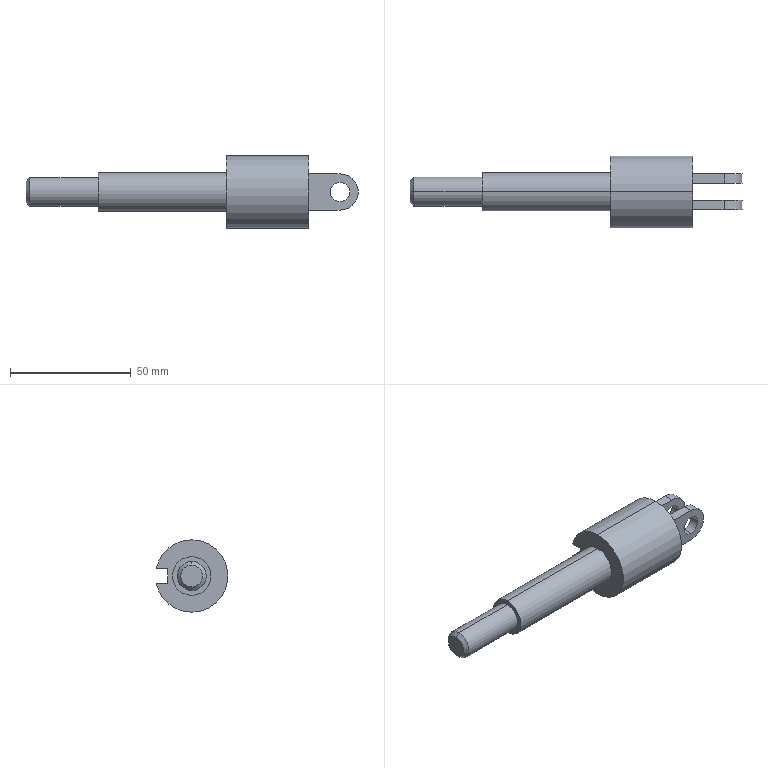Part | SolidWorks | features MirrorStock 1 | 1 solid | 30 faces | box 137.5 x 29.697 x 30 mm | volume 38909 mm3 | plane 15 | cylinder 13 | cone 2 | commonest cylinder face diameters 8 x4 30 x3 12 x2 15 x2 16 x2
STEP:
#1=CARTESIAN_POINT('',(30.,-7.5,-4.));
#2=VERTEX_POINT('',#1);
#3=CARTESIAN_POINT('',(30.,-7.5,4.));
#4=VERTEX_POINT('',#3);
#5=CARTESIAN_POINT('',(30.,-7.5,0.));
#6=DIRECTION('',(0.,-1.,0.));
#7=DIRECTION('',(0.,0.,-1.));
#8=AXIS2_PLACEMENT_3D('',#5,#6,#7);
#9=CIRCLE('',#8,4.);
#10=EDGE_CURVE('',#2,#4,#9,.T.);
#11=ORIENTED_EDGE('',*,*,#10,.T.);
#12=CARTESIAN_POINT('',(30.,-3.5,4.));
#13=VERTEX_POINT('',#12);
#14=CARTESIAN_POINT('',(30.,-7.5,4.));
#15=DIRECTION('',(0.,1.,0.));
#16=VECTOR('',#15,1000.);
#17=LINE('',#14,#16);
#18=EDGE_CURVE('',#4,#13,#17,.T.);
#19=ORIENTED_EDGE('',*,*,#18,.T.);
#20=CARTESIAN_POINT('',(30.,-3.5,-4.));
#21=VERTEX_POINT('',#20);
#22=CARTESIAN_POINT('',(30.,-3.5,0.));
#23=DIRECTION('',(0.,-1.,0.));
#24=DIRECTION('',(0.,0.,-1.));
#25=AXIS2_PLACEMENT_3D('',#22,#23,#24);
#26=CIRCLE('',#25,4.);
#27=EDGE_CURVE('',#21,#13,#26,.T.);
#28=ORIENTED_EDGE('',*,*,#27,.F.);
#29=CARTESIAN_POINT('',(30.,-7.5,-4.));
#30=DIRECTION('',(0.,1.,0.));
#31=VECTOR('',#30,1000.);
#32=LINE('',#29,#31);
#33=EDGE_CURVE('',#2,#21,#32,.T.);
#34=ORIENTED_EDGE('',*,*,#33,.F.);
#35=EDGE_LOOP('',(#11,#19,#28,#34));
#36=FACE_OUTER_BOUND('',#35,.T.);
#37=CARTESIAN_POINT('',(30.,-7.5,0.));
#38=DIRECTION('',(0.,1.,0.));
#39=DIRECTION('',(0.,0.,-1.));
#40=AXIS2_PLACEMENT_3D('',#37,#38,#39);
#41=CYLINDRICAL_SURFACE('',#40,4.);
#42=ADVANCED_FACE('',(#36),#41,.F.);
#43=CARTESIAN_POINT('',(30.,7.5,-4.));
#44=VERTEX_POINT('',#43);
#45=CARTESIAN_POINT('',(30.,7.5,4.));
#46=VERTEX_POINT('',#45);
#47=CARTESIAN_POINT('',(30.,7.5,0.));
#48=DIRECTION('',(0.,-1.,0.));
#49=DIRECTION('',(0.,0.,-1.));
#50=AXIS2_PLACEMENT_3D('',#47,#48,#49);
#51=CIRCLE('',#50,4.);
#52=EDGE_CURVE('',#44,#46,#51,.T.);
#53=ORIENTED_EDGE('',*,*,#52,.F.);
#54=CARTESIAN_POINT('',(30.,3.5,-4.));
#55=VERTEX_POINT('',#54);
#56=CARTESIAN_POINT('',(30.,7.5,-4.));
#57=DIRECTION('',(0.,-1.,0.));
#58=VECTOR('',#57,1000.);
#59=LINE('',#56,#58);
#60=EDGE_CURVE('',#44,#55,#59,.T.);
#61=ORIENTED_EDGE('',*,*,#60,.T.);
#62=CARTESIAN_POINT('',(30.,3.5,4.));
#63=VERTEX_POINT('',#62);
#64=CARTESIAN_POINT('',(30.,3.5,0.));
#65=DIRECTION('',(0.,-1.,0.));
#66=DIRECTION('',(0.,0.,-1.));
#67=AXIS2_PLACEMENT_3D('',#64,#65,#66);
#68=CIRCLE('',#67,4.);
#69=EDGE_CURVE('',#55,#63,#68,.T.);
#70=ORIENTED_EDGE('',*,*,#69,.T.);
#71=CARTESIAN_POINT('',(30.,7.5,4.));
#72=DIRECTION('',(0.,-1.,0.));
#73=VECTOR('',#72,1000.);
#74=LINE('',#71,#73);
#75=EDGE_CURVE('',#46,#63,#74,.T.);
#76=ORIENTED_EDGE('',*,*,#75,.F.);
#77=EDGE_LOOP('',(#53,#61,#70,#76));
#78=FACE_OUTER_BOUND('',#77,.T.);
#79=CARTESIAN_POINT('',(30.,7.5,0.));
#80=DIRECTION('',(0.,-1.,0.));
#81=DIRECTION('',(0.,0.,1.));
#82=AXIS2_PLACEMENT_3D('',#79,#80,#81);
#83=CYLINDRICAL_SURFACE('',#82,4.);
#84=ADVANCED_FACE('',(#78),#83,.F.);
#85=CARTESIAN_POINT('',(-100.,0.,4.5));
#86=VERTEX_POINT('',#85);
#87=CARTESIAN_POINT('',(-100.,0.,-4.5));
#88=VERTEX_POINT('',#87);
#89=CARTESIAN_POINT('',(-100.,0.,0.));
#90=DIRECTION('',(1.,0.,0.));
#91=DIRECTION('',(0.,0.,-1.));
#92=AXIS2_PLACEMENT_3D('',#89,#90,#91);
#93=CIRCLE('',#92,4.5);
#94=EDGE_CURVE('',#86,#88,#93,.T.);
#95=ORIENTED_EDGE('',*,*,#94,.T.);
#96=CARTESIAN_POINT('',(-98.5,0.,-6.));
#97=VERTEX_POINT('',#96);
#98=CARTESIAN_POINT('',(-100.,0.,-4.5));
#99=DIRECTION('',(0.7071,0.,-0.7071));
#100=VECTOR('',#99,1000.);
#101=LINE('',#98,#100);
#102=EDGE_CURVE('',#88,#97,#101,.T.);
#103=ORIENTED_EDGE('',*,*,#102,.T.);
#104=CARTESIAN_POINT('',(-98.5,0.,6.));
#105=VERTEX_POINT('',#104);
#106=CARTESIAN_POINT('',(-98.5,0.,0.));
#107=DIRECTION('',(-1.,0.,0.));
#108=DIRECTION('',(0.,0.,-1.));
#109=AXIS2_PLACEMENT_3D('',#106,#107,#108);
#110=CIRCLE('',#109,6.);
#111=EDGE_CURVE('',#97,#105,#110,.T.);
#112=ORIENTED_EDGE('',*,*,#111,.T.);
#113=CARTESIAN_POINT('',(-100.,0.,4.5));
#114=DIRECTION('',(0.7071,0.,0.7071));
#115=VECTOR('',#114,1000.);
#116=LINE('',#113,#115);
#117=EDGE_CURVE('',#86,#105,#116,.T.);
#118=ORIENTED_EDGE('',*,*,#117,.F.);
#119=EDGE_LOOP('',(#95,#103,#112,#118));
#120=FACE_OUTER_BOUND('',#119,.T.);
#121=CARTESIAN_POINT('',(-100.,0.,0.));
#122=DIRECTION('',(1.,0.,0.));
#123=DIRECTION('',(0.,0.,1.));
#124=AXIS2_PLACEMENT_3D('',#121,#122,#123);
#125=CONICAL_SURFACE('',#124,4.5,0.7854);
#126=ADVANCED_FACE('',(#120),#125,.T.);
#127=ORIENTED_EDGE('',*,*,#111,.F.);
#128=CARTESIAN_POINT('',(-70.,0.,-6.));
#129=VERTEX_POINT('',#128);
#130=CARTESIAN_POINT('',(-100.,0.,-6.));
#131=DIRECTION('',(1.,0.,0.));
#132=VECTOR('',#131,1000.);
#133=LINE('',#130,#132);
#134=EDGE_CURVE('',#97,#129,#133,.T.);
#135=ORIENTED_EDGE('',*,*,#134,.T.);
#136=CARTESIAN_POINT('',(-70.,0.,6.));
#137=VERTEX_POINT('',#136);
#138=CARTESIAN_POINT('',(-70.,0.,0.));
#139=DIRECTION('',(1.,0.,0.));
#140=DIRECTION('',(0.,0.,-1.));
#141=AXIS2_PLACEMENT_3D('',#138,#139,#140);
#142=CIRCLE('',#141,6.);
#143=EDGE_CURVE('',#137,#129,#142,.T.);
#144=ORIENTED_EDGE('',*,*,#143,.F.);
#145=CARTESIAN_POINT('',(-100.,0.,6.));
#146=DIRECTION('',(1.,0.,0.));
#147=VECTOR('',#146,1000.);
#148=LINE('',#145,#147);
#149=EDGE_CURVE('',#105,#137,#148,.T.);
#150=ORIENTED_EDGE('',*,*,#149,.F.);
#151=EDGE_LOOP('',(#127,#135,#144,#150));
#152=FACE_OUTER_BOUND('',#151,.T.);
#153=CARTESIAN_POINT('',(-100.,0.,0.));
#154=DIRECTION('',(1.,0.,0.));
#155=DIRECTION('',(0.,0.,1.));
#156=AXIS2_PLACEMENT_3D('',#153,#154,#155);
#157=CYLINDRICAL_SURFACE('',#156,6.);
#158=ADVANCED_FACE('',(#152),#157,.T.);
#159=CARTESIAN_POINT('',(-70.,0.,8.));
#160=VERTEX_POINT('',#159);
#161=CARTESIAN_POINT('',(-70.,0.,-8.));
#162=VERTEX_POINT('',#161);
#163=CARTESIAN_POINT('',(-70.,0.,0.));
#164=DIRECTION('',(1.,0.,0.));
#165=DIRECTION('',(0.,0.,-1.));
#166=AXIS2_PLACEMENT_3D('',#163,#164,#165);
#167=CIRCLE('',#166,8.);
#168=EDGE_CURVE('',#160,#162,#167,.T.);
#169=ORIENTED_EDGE('',*,*,#168,.T.);
#170=CARTESIAN_POINT('',(-17.,0.,-8.));
#171=VERTEX_POINT('',#170);
#172=CARTESIAN_POINT('',(-70.,0.,-8.));
#173=DIRECTION('',(1.,0.,0.));
#174=VECTOR('',#173,1000.);
#175=LINE('',#172,#174);
#176=EDGE_CURVE('',#162,#171,#175,.T.);
#177=ORIENTED_EDGE('',*,*,#176,.T.);
#178=CARTESIAN_POINT('',(-17.,0.,8.));
#179=VERTEX_POINT('',#178);
#180=CARTESIAN_POINT('',(-17.,0.,0.));
#181=DIRECTION('',(1.,0.,0.));
#182=DIRECTION('',(0.,0.,1.));
#183=AXIS2_PLACEMENT_3D('',#180,#181,#182);
#184=CIRCLE('',#183,8.);
#185=EDGE_CURVE('',#179,#171,#184,.T.);
#186=ORIENTED_EDGE('',*,*,#185,.F.);
#187=CARTESIAN_POINT('',(-70.,0.,8.));
#188=DIRECTION('',(1.,0.,0.));
#189=VECTOR('',#188,1000.);
#190=LINE('',#187,#189);
#191=EDGE_CURVE('',#160,#179,#190,.T.);
#192=ORIENTED_EDGE('',*,*,#191,.F.);
#193=EDGE_LOOP('',(#169,#177,#186,#192));
#194=FACE_OUTER_BOUND('',#193,.T.);
#195=CARTESIAN_POINT('',(-70.,0.,0.));
#196=DIRECTION('',(1.,0.,0.));
#197=DIRECTION('',(0.,0.,1.));
#198=AXIS2_PLACEMENT_3D('',#195,#196,#197);
#199=CYLINDRICAL_SURFACE('',#198,8.);
#200=ADVANCED_FACE('',(#194),#199,.T.);
#201=CARTESIAN_POINT('',(-17.,0.,15.));
#202=VERTEX_POINT('',#201);
#203=CARTESIAN_POINT('',(-17.,0.,-15.));
#204=VERTEX_POINT('',#203);
#205=CARTESIAN_POINT('',(-17.,0.,0.));
#206=DIRECTION('',(1.,0.,0.));
#207=DIRECTION('',(0.,0.,1.));
#208=AXIS2_PLACEMENT_3D('',#205,#206,#207);
#209=CIRCLE('',#208,15.);
#210=EDGE_CURVE('',#202,#204,#209,.T.);
#211=ORIENTED_EDGE('',*,*,#210,.T.);
#212=CARTESIAN_POINT('',(17.,0.,-15.));
#213=VERTEX_POINT('',#212);
#214=CARTESIAN_POINT('',(-87.711,0.,-15.));
#215=DIRECTION('',(1.,0.,0.));
#216=VECTOR('',#215,1000.);
#217=LINE('',#214,#216);
#218=EDGE_CURVE('',#204,#213,#217,.T.);
#219=ORIENTED_EDGE('',*,*,#218,.T.);
#220=CARTESIAN_POINT('',(17.,0.,15.));
#221=VERTEX_POINT('',#220);
#222=CARTESIAN_POINT('',(17.,0.,0.));
#223=DIRECTION('',(-1.,0.,0.));
#224=DIRECTION('',(0.,0.,1.));
#225=AXIS2_PLACEMENT_3D('',#222,#223,#224);
#226=CIRCLE('',#225,15.);
#227=EDGE_CURVE('',#213,#221,#226,.T.);
#228=ORIENTED_EDGE('',*,*,#227,.T.);
#229=CARTESIAN_POINT('',(-87.711,0.,15.));
#230=DIRECTION('',(1.,0.,0.));
#231=VECTOR('',#230,1000.);
#232=LINE('',#229,#231);
#233=EDGE_CURVE('',#202,#221,#232,.T.);
#234=ORIENTED_EDGE('',*,*,#233,.F.);
#235=EDGE_LOOP('',(#211,#219,#228,#234));
#236=FACE_OUTER_BOUND('',#235,.T.);
#237=CARTESIAN_POINT('',(-87.711,0.,0.));
#238=DIRECTION('',(1.,0.,0.));
#239=DIRECTION('',(0.,0.,1.));
#240=AXIS2_PLACEMENT_3D('',#237,#238,#239);
#241=CYLINDRICAL_SURFACE('',#240,15.);
#242=ADVANCED_FACE('',(#236),#241,.T.);
#243=CARTESIAN_POINT('',(-17.,14.697,3.));
#244=VERTEX_POINT('',#243);
#245=CARTESIAN_POINT('',(-17.,0.,0.));
#246=DIRECTION('',(1.,0.,0.));
#247=DIRECTION('',(0.,0.,1.));
#248=AXIS2_PLACEMENT_3D('',#245,#246,#247);
#249=CIRCLE('',#248,15.);
#250=EDGE_CURVE('',#244,#202,#249,.T.);
#251=ORIENTED_EDGE('',*,*,#250,.T.);
#252=ORIENTED_EDGE('',*,*,#233,.T.);
#253=CARTESIAN_POINT('',(17.,14.697,3.));
#254=VERTEX_POINT('',#253);
#255=CARTESIAN_POINT('',(17.,0.,0.));
#256=DIRECTION('',(-1.,0.,0.));
#257=DIRECTION('',(0.,0.,1.));
#258=AXIS2_PLACEMENT_3D('',#255,#256,#257);
#259=CIRCLE('',#258,15.);
#260=EDGE_CURVE('',#221,#254,#259,.T.);
#261=ORIENTED_EDGE('',*,*,#260,.T.);
#262=CARTESIAN_POINT('',(-87.711,14.697,3.));
#263=DIRECTION('',(1.,0.,0.));
#264=VECTOR('',#263,1000.);
#265=LINE('',#262,#264);
#266=EDGE_CURVE('',#244,#254,#265,.T.);
#267=ORIENTED_EDGE('',*,*,#266,.F.);
#268=EDGE_LOOP('',(#251,#252,#261,#267));
#269=FACE_OUTER_BOUND('',#268,.T.);
#270=CARTESIAN_POINT('',(-87.711,0.,0.));
#271=DIRECTION('',(1.,0.,0.));
#272=DIRECTION('',(0.,0.,1.));
#273=AXIS2_PLACEMENT_3D('',#270,#271,#272);
#274=CYLINDRICAL_SURFACE('',#273,15.);
#275=ADVANCED_FACE('',(#269),#274,.T.);
#276=CARTESIAN_POINT('',(17.,-7.5,7.5));
#277=VERTEX_POINT('',#276);
#278=CARTESIAN_POINT('',(17.,-3.5,7.5));
#279=VERTEX_POINT('',#278);
#280=CARTESIAN_POINT('',(17.,-7.5,7.5));
#281=DIRECTION('',(0.,1.,0.));
#282=VECTOR('',#281,1000.);
#283=LINE('',#280,#282);
#284=EDGE_CURVE('',#277,#279,#283,.T.);
#285=ORIENTED_EDGE('',*,*,#284,.T.);
#286=CARTESIAN_POINT('',(17.,-3.5,-7.5));
#287=VERTEX_POINT('',#286);
#288=CARTESIAN_POINT('',(17.,-3.5,-7.5));
#289=DIRECTION('',(0.,0.,-1.));
#290=VECTOR('',#289,1000.);
#291=LINE('',#288,#290);
#292=EDGE_CURVE('',#279,#287,#291,.T.);
#293=ORIENTED_EDGE('',*,*,#292,.T.);
#294=CARTESIAN_POINT('',(17.,-7.5,-7.5));
#295=VERTEX_POINT('',#294);
#296=CARTESIAN_POINT('',(17.,-7.5,-7.5));
#297=DIRECTION('',(0.,1.,0.));
#298=VECTOR('',#297,1000.);
#299=LINE('',#296,#298);
#300=EDGE_CURVE('',#295,#287,#299,.T.);
#301=ORIENTED_EDGE('',*,*,#300,.F.);
#302=CARTESIAN_POINT('',(17.,-7.5,-7.5));
#303=DIRECTION('',(0.,0.,-1.));
#304=VECTOR('',#303,1000.);
#305=LINE('',#302,#304);
#306=EDGE_CURVE('',#277,#295,#305,.T.);
#307=ORIENTED_EDGE('',*,*,#306,.F.);
#308=EDGE_LOOP('',(#285,#293,#301,#307));
#309=FACE_BOUND('',#308,.T.);
#310=CARTESIAN_POINT('',(17.,10.,3.));
#311=VERTEX_POINT('',#310);
#312=CARTESIAN_POINT('',(17.,15.,3.));
#313=DIRECTION('',(0.,-1.,0.));
#314=VECTOR('',#313,1000.);
#315=LINE('',#312,#314);
#316=EDGE_CURVE('',#254,#311,#315,.T.);
#317=ORIENTED_EDGE('',*,*,#316,.F.);
#318=ORIENTED_EDGE('',*,*,#260,.F.);
#319=ORIENTED_EDGE('',*,*,#227,.F.);
#320=CARTESIAN_POINT('',(17.,14.697,-3.));
#321=VERTEX_POINT('',#320);
#322=CARTESIAN_POINT('',(17.,0.,0.));
#323=DIRECTION('',(-1.,0.,0.));
#324=DIRECTION('',(0.,0.,1.));
#325=AXIS2_PLACEMENT_3D('',#322,#323,#324);
#326=CIRCLE('',#325,15.);
#327=EDGE_CURVE('',#321,#213,#326,.T.);
#328=ORIENTED_EDGE('',*,*,#327,.F.);
#329=CARTESIAN_POINT('',(17.,10.,-3.));
#330=VERTEX_POINT('',#329);
#331=CARTESIAN_POINT('',(17.,15.,-3.));
#332=DIRECTION('',(0.,-1.,0.));
#333=VECTOR('',#332,1000.);
#334=LINE('',#331,#333);
#335=EDGE_CURVE('',#321,#330,#334,.T.);
#336=ORIENTED_EDGE('',*,*,#335,.T.);
#337=CARTESIAN_POINT('',(17.,10.,-3.));
#338=DIRECTION('',(0.,0.,1.));
#339=VECTOR('',#338,1000.);
#340=LINE('',#337,#339);
#341=EDGE_CURVE('',#330,#311,#340,.T.);
#342=ORIENTED_EDGE('',*,*,#341,.T.);
#343=EDGE_LOOP('',(#317,#318,#319,#328,#336,#342));
#344=FACE_OUTER_BOUND('',#343,.T.);
#345=CARTESIAN_POINT('',(17.,7.5,-7.5));
#346=VERTEX_POINT('',#345);
#347=CARTESIAN_POINT('',(17.,3.5,-7.5));
#348=VERTEX_POINT('',#347);
#349=CARTESIAN_POINT('',(17.,7.5,-7.5));
#350=DIRECTION('',(0.,-1.,0.));
#351=VECTOR('',#350,1000.);
#352=LINE('',#349,#351);
#353=EDGE_CURVE('',#346,#348,#352,.T.);
#354=ORIENTED_EDGE('',*,*,#353,.T.);
#355=CARTESIAN_POINT('',(17.,3.5,7.5));
#356=VERTEX_POINT('',#355);
#357=CARTESIAN_POINT('',(17.,3.5,-7.5));
#358=DIRECTION('',(0.,0.,-1.));
#359=VECTOR('',#358,1000.);
#360=LINE('',#357,#359);
#361=EDGE_CURVE('',#356,#348,#360,.T.);
#362=ORIENTED_EDGE('',*,*,#361,.F.);
#363=CARTESIAN_POINT('',(17.,7.5,7.5));
#364=VERTEX_POINT('',#363);
#365=CARTESIAN_POINT('',(17.,7.5,7.5));
#366=DIRECTION('',(0.,-1.,0.));
#367=VECTOR('',#366,1000.);
#368=LINE('',#365,#367);
#369=EDGE_CURVE('',#364,#356,#368,.T.);
#370=ORIENTED_EDGE('',*,*,#369,.F.);
#371=CARTESIAN_POINT('',(17.,7.5,-7.5));
#372=DIRECTION('',(0.,0.,-1.));
#373=VECTOR('',#372,1000.);
#374=LINE('',#371,#373);
#375=EDGE_CURVE('',#364,#346,#374,.T.);
#376=ORIENTED_EDGE('',*,*,#375,.T.);
#377=EDGE_LOOP('',(#354,#362,#370,#376));
#378=FACE_BOUND('',#377,.T.);
#379=CARTESIAN_POINT('',(17.,-15.,-15.));
#380=DIRECTION('',(-1.,0.,0.));
#381=DIRECTION('',(0.,0.,-1.));
#382=AXIS2_PLACEMENT_3D('',#379,#380,#381);
#383=PLANE('',#382);
#384=ADVANCED_FACE('',(#309,#344,#378),#383,.F.);
#385=ORIENTED_EDGE('',*,*,#218,.F.);
#386=CARTESIAN_POINT('',(-17.,14.697,-3.));
#387=VERTEX_POINT('',#386);
#388=CARTESIAN_POINT('',(-17.,0.,0.));
#389=DIRECTION('',(1.,0.,0.));
#390=DIRECTION('',(0.,0.,1.));
#391=AXIS2_PLACEMENT_3D('',#388,#389,#390);
#392=CIRCLE('',#391,15.);
#393=EDGE_CURVE('',#204,#387,#392,.T.);
#394=ORIENTED_EDGE('',*,*,#393,.T.);
#395=CARTESIAN_POINT('',(-87.711,14.697,-3.));
#396=DIRECTION('',(-1.,0.,0.));
#397=VECTOR('',#396,1000.);
#398=LINE('',#395,#397);
#399=EDGE_CURVE('',#321,#387,#398,.T.);
#400=ORIENTED_EDGE('',*,*,#399,.F.);
#401=ORIENTED_EDGE('',*,*,#327,.T.);
#402=EDGE_LOOP('',(#385,#394,#400,#401));
#403=FACE_OUTER_BOUND('',#402,.T.);
#404=CARTESIAN_POINT('',(-87.711,0.,0.));
#405=DIRECTION('',(1.,0.,0.));
#406=DIRECTION('',(0.,0.,1.));
#407=AXIS2_PLACEMENT_3D('',#404,#405,#406);
#408=CYLINDRICAL_SURFACE('',#407,15.);
#409=ADVANCED_FACE('',(#403),#408,.T.);
#410=ORIENTED_EDGE('',*,*,#185,.T.);
#411=CARTESIAN_POINT('',(-17.,0.,0.));
#412=DIRECTION('',(1.,0.,0.));
#413=DIRECTION('',(0.,0.,1.));
#414=AXIS2_PLACEMENT_3D('',#411,#412,#413);
#415=CIRCLE('',#414,8.);
#416=EDGE_CURVE('',#171,#179,#415,.T.);
#417=ORIENTED_EDGE('',*,*,#416,.T.);
#418=EDGE_LOOP('',(#410,#417));
#419=FACE_BOUND('',#418,.T.);
#420=CARTESIAN_POINT('',(-17.,10.,3.));
#421=VERTEX_POINT('',#420);
#422=CARTESIAN_POINT('',(-17.,-15.,3.));
#423=DIRECTION('',(0.,-1.,0.));
#424=VECTOR('',#423,1000.);
#425=LINE('',#422,#424);
#426=EDGE_CURVE('',#244,#421,#425,.T.);
#427=ORIENTED_EDGE('',*,*,#426,.T.);
#428=CARTESIAN_POINT('',(-17.,10.,-3.));
#429=VERTEX_POINT('',#428);
#430=CARTESIAN_POINT('',(-17.,10.,-3.));
#431=DIRECTION('',(0.,0.,-1.));
#432=VECTOR('',#431,1000.);
#433=LINE('',#430,#432);
#434=EDGE_CURVE('',#421,#429,#433,.T.);
#435=ORIENTED_EDGE('',*,*,#434,.T.);
#436=CARTESIAN_POINT('',(-17.,-15.,-3.));
#437=DIRECTION('',(0.,1.,0.));
#438=VECTOR('',#437,1000.);
#439=LINE('',#436,#438);
#440=EDGE_CURVE('',#429,#387,#439,.T.);
#441=ORIENTED_EDGE('',*,*,#440,.T.);
#442=ORIENTED_EDGE('',*,*,#393,.F.);
#443=ORIENTED_EDGE('',*,*,#210,.F.);
#444=ORIENTED_EDGE('',*,*,#250,.F.);
#445=EDGE_LOOP('',(#427,#435,#441,#442,#443,#444));
#446=FACE_OUTER_BOUND('',#445,.T.);
#447=CARTESIAN_POINT('',(-17.,-15.,-15.));
#448=DIRECTION('',(1.,0.,0.));
#449=DIRECTION('',(0.,0.,1.));
#450=AXIS2_PLACEMENT_3D('',#447,#448,#449);
#451=PLANE('',#450);
#452=ADVANCED_FACE('',(#419,#446),#451,.F.);
#453=ORIENTED_EDGE('',*,*,#426,.F.);
#454=ORIENTED_EDGE('',*,*,#266,.T.);
#455=ORIENTED_EDGE('',*,*,#316,.T.);
#456=CARTESIAN_POINT('',(-17.,10.,3.));
#457=DIRECTION('',(-1.,0.,0.));
#458=VECTOR('',#457,1000.);
#459=LINE('',#456,#458);
#460=EDGE_CURVE('',#311,#421,#459,.T.);
#461=ORIENTED_EDGE('',*,*,#460,.T.);
#462=EDGE_LOOP('',(#453,#454,#455,#461));
#463=FACE_OUTER_BOUND('',#462,.T.);
#464=CARTESIAN_POINT('',(-17.,15.,3.));
#465=DIRECTION('',(0.,0.,-1.));
#466=DIRECTION('',(1.,0.,0.));
#467=AXIS2_PLACEMENT_3D('',#464,#465,#466);
#468=PLANE('',#467);
#469=ADVANCED_FACE('',(#463),#468,.T.);
#470=ORIENTED_EDGE('',*,*,#335,.F.);
#471=ORIENTED_EDGE('',*,*,#399,.T.);
#472=ORIENTED_EDGE('',*,*,#440,.F.);
#473=CARTESIAN_POINT('',(-17.,10.,-3.));
#474=DIRECTION('',(1.,0.,0.));
#475=VECTOR('',#474,1000.);
#476=LINE('',#473,#475);
#477=EDGE_CURVE('',#429,#330,#476,.T.);
#478=ORIENTED_EDGE('',*,*,#477,.T.);
#479=EDGE_LOOP('',(#470,#471,#472,#478));
#480=FACE_OUTER_BOUND('',#479,.T.);
#481=CARTESIAN_POINT('',(-17.,15.,-3.));
#482=DIRECTION('',(0.,0.,1.));
#483=DIRECTION('',(-1.,0.,0.));
#484=AXIS2_PLACEMENT_3D('',#481,#482,#483);
#485=PLANE('',#484);
#486=ADVANCED_FACE('',(#480),#485,.T.);
#487=ORIENTED_EDGE('',*,*,#341,.F.);
#488=ORIENTED_EDGE('',*,*,#477,.F.);
#489=ORIENTED_EDGE('',*,*,#434,.F.);
#490=ORIENTED_EDGE('',*,*,#460,.F.);
#491=EDGE_LOOP('',(#487,#488,#489,#490));
#492=FACE_OUTER_BOUND('',#491,.T.);
#493=CARTESIAN_POINT('',(0.,10.,0.));
#494=DIRECTION('',(0.,-1.,0.));
#495=DIRECTION('',(0.,0.,1.));
#496=AXIS2_PLACEMENT_3D('',#493,#494,#495);
#497=PLANE('',#496);
#498=ADVANCED_FACE('',(#492),#497,.F.);
#499=ORIENTED_EDGE('',*,*,#176,.F.);
#500=CARTESIAN_POINT('',(-70.,0.,0.));
#501=DIRECTION('',(1.,0.,0.));
#502=DIRECTION('',(0.,0.,-1.));
#503=AXIS2_PLACEMENT_3D('',#500,#501,#502);
#504=CIRCLE('',#503,8.);
#505=EDGE_CURVE('',#162,#160,#504,.T.);
#506=ORIENTED_EDGE('',*,*,#505,.T.);
#507=ORIENTED_EDGE('',*,*,#191,.T.);
#508=ORIENTED_EDGE('',*,*,#416,.F.);
#509=EDGE_LOOP('',(#499,#506,#507,#508));
#510=FACE_OUTER_BOUND('',#509,.T.);
#511=CARTESIAN_POINT('',(-70.,0.,0.));
#512=DIRECTION('',(1.,0.,0.));
#513=DIRECTION('',(0.,0.,1.));
#514=AXIS2_PLACEMENT_3D('',#511,#512,#513);
#515=CYLINDRICAL_SURFACE('',#514,8.);
#516=ADVANCED_FACE('',(#510),#515,.T.);
#517=ORIENTED_EDGE('',*,*,#143,.T.);
#518=CARTESIAN_POINT('',(-70.,0.,0.));
#519=DIRECTION('',(1.,0.,0.));
#520=DIRECTION('',(0.,0.,-1.));
#521=AXIS2_PLACEMENT_3D('',#518,#519,#520);
#522=CIRCLE('',#521,6.);
#523=EDGE_CURVE('',#129,#137,#522,.T.);
#524=ORIENTED_EDGE('',*,*,#523,.T.);
#525=EDGE_LOOP('',(#517,#524));
#526=FACE_BOUND('',#525,.T.);
#527=ORIENTED_EDGE('',*,*,#168,.F.);
#528=ORIENTED_EDGE('',*,*,#505,.F.);
#529=EDGE_LOOP('',(#527,#528));
#530=FACE_OUTER_BOUND('',#529,.T.);
#531=CARTESIAN_POINT('',(-70.,0.,0.));
#532=DIRECTION('',(-1.,0.,0.));
#533=DIRECTION('',(0.,0.,-1.));
#534=AXIS2_PLACEMENT_3D('',#531,#532,#533);
#535=PLANE('',#534);
#536=ADVANCED_FACE('',(#526,#530),#535,.T.);
#537=ORIENTED_EDGE('',*,*,#134,.F.);
#538=CARTESIAN_POINT('',(-98.5,0.,0.));
#539=DIRECTION('',(-1.,0.,0.));
#540=DIRECTION('',(0.,0.,-1.));
#541=AXIS2_PLACEMENT_3D('',#538,#539,#540);
#542=CIRCLE('',#541,6.);
#543=EDGE_CURVE('',#105,#97,#542,.T.);
#544=ORIENTED_EDGE('',*,*,#543,.F.);
#545=ORIENTED_EDGE('',*,*,#149,.T.);
#546=ORIENTED_EDGE('',*,*,#523,.F.);
#547=EDGE_LOOP('',(#537,#544,#545,#546));
#548=FACE_OUTER_BOUND('',#547,.T.);
#549=CARTESIAN_POINT('',(-100.,0.,0.));
#550=DIRECTION('',(1.,0.,0.));
#551=DIRECTION('',(0.,0.,1.));
#552=AXIS2_PLACEMENT_3D('',#549,#550,#551);
#553=CYLINDRICAL_SURFACE('',#552,6.);
#554=ADVANCED_FACE('',(#548),#553,.T.);
#555=ORIENTED_EDGE('',*,*,#94,.F.);
#556=CARTESIAN_POINT('',(-100.,0.,0.));
#557=DIRECTION('',(1.,0.,0.));
#558=DIRECTION('',(0.,0.,-1.));
#559=AXIS2_PLACEMENT_3D('',#556,#557,#558);
#560=CIRCLE('',#559,4.5);
#561=EDGE_CURVE('',#88,#86,#560,.T.);
#562=ORIENTED_EDGE('',*,*,#561,.F.);
#563=EDGE_LOOP('',(#555,#562));
#564=FACE_OUTER_BOUND('',#563,.T.);
#565=CARTESIAN_POINT('',(-100.,0.,0.));
#566=DIRECTION('',(-1.,0.,0.));
#567=DIRECTION('',(0.,0.,-1.));
#568=AXIS2_PLACEMENT_3D('',#565,#566,#567);
#569=PLANE('',#568);
#570=ADVANCED_FACE('',(#564),#569,.T.);
#571=ORIENTED_EDGE('',*,*,#102,.F.);
#572=ORIENTED_EDGE('',*,*,#561,.T.);
#573=ORIENTED_EDGE('',*,*,#117,.T.);
#574=ORIENTED_EDGE('',*,*,#543,.T.);
#575=EDGE_LOOP('',(#571,#572,#573,#574));
#576=FACE_OUTER_BOUND('',#575,.T.);
#577=CARTESIAN_POINT('',(-100.,0.,0.));
#578=DIRECTION('',(1.,0.,0.));
#579=DIRECTION('',(0.,0.,1.));
#580=AXIS2_PLACEMENT_3D('',#577,#578,#579);
#581=CONICAL_SURFACE('',#580,4.5,0.7854);
#582=ADVANCED_FACE('',(#576),#581,.T.);
#583=ORIENTED_EDGE('',*,*,#375,.F.);
#584=CARTESIAN_POINT('',(30.,7.5,7.5));
#585=VERTEX_POINT('',#584);
#586=CARTESIAN_POINT('',(30.,7.5,7.5));
#587=DIRECTION('',(-1.,0.,0.));
#588=VECTOR('',#587,1000.);
#589=LINE('',#586,#588);
#590=EDGE_CURVE('',#585,#364,#589,.T.);
#591=ORIENTED_EDGE('',*,*,#590,.F.);
#592=CARTESIAN_POINT('',(30.,7.5,-7.5));
#593=VERTEX_POINT('',#592);
#594=CARTESIAN_POINT('',(30.,7.5,0.));
#595=DIRECTION('',(0.,-1.,0.));
#596=DIRECTION('',(0.,0.,-1.));
#597=AXIS2_PLACEMENT_3D('',#594,#595,#596);
#598=CIRCLE('',#597,7.5);
#599=EDGE_CURVE('',#593,#585,#598,.T.);
#600=ORIENTED_EDGE('',*,*,#599,.F.);
#601=CARTESIAN_POINT('',(30.,7.5,-7.5));
#602=DIRECTION('',(1.,0.,0.));
#603=VECTOR('',#602,1000.);
#604=LINE('',#601,#603);
#605=EDGE_CURVE('',#346,#593,#604,.T.);
#606=ORIENTED_EDGE('',*,*,#605,.F.);
#607=EDGE_LOOP('',(#583,#591,#600,#606));
#608=FACE_OUTER_BOUND('',#607,.T.);
#609=CARTESIAN_POINT('',(30.,7.5,0.));
#610=DIRECTION('',(0.,-1.,0.));
#611=DIRECTION('',(0.,0.,-1.));
#612=AXIS2_PLACEMENT_3D('',#609,#610,#611);
#613=CIRCLE('',#612,4.);
#614=EDGE_CURVE('',#46,#44,#613,.T.);
#615=ORIENTED_EDGE('',*,*,#614,.T.);
#616=ORIENTED_EDGE('',*,*,#52,.T.);
#617=EDGE_LOOP('',(#615,#616));
#618=FACE_BOUND('',#617,.T.);
#619=CARTESIAN_POINT('',(30.,7.5,0.));
#620=DIRECTION('',(0.,1.,0.));
#621=DIRECTION('',(0.,0.,-1.));
#622=AXIS2_PLACEMENT_3D('',#619,#620,#621);
#623=PLANE('',#622);
#624=ADVANCED_FACE('',(#608,#618),#623,.T.);
#625=ORIENTED_EDGE('',*,*,#361,.T.);
#626=CARTESIAN_POINT('',(30.,3.5,-7.5));
#627=VERTEX_POINT('',#626);
#628=CARTESIAN_POINT('',(30.,3.5,-7.5));
#629=DIRECTION('',(1.,0.,0.));
#630=VECTOR('',#629,1000.);
#631=LINE('',#628,#630);
#632=EDGE_CURVE('',#348,#627,#631,.T.);
#633=ORIENTED_EDGE('',*,*,#632,.T.);
#634=CARTESIAN_POINT('',(30.,3.5,7.5));
#635=VERTEX_POINT('',#634);
#636=CARTESIAN_POINT('',(30.,3.5,0.));
#637=DIRECTION('',(0.,-1.,0.));
#638=DIRECTION('',(0.,0.,-1.));
#639=AXIS2_PLACEMENT_3D('',#636,#637,#638);
#640=CIRCLE('',#639,7.5);
#641=EDGE_CURVE('',#627,#635,#640,.T.);
#642=ORIENTED_EDGE('',*,*,#641,.T.);
#643=CARTESIAN_POINT('',(30.,3.5,7.5));
#644=DIRECTION('',(-1.,0.,0.));
#645=VECTOR('',#644,1000.);
#646=LINE('',#643,#645);
#647=EDGE_CURVE('',#635,#356,#646,.T.);
#648=ORIENTED_EDGE('',*,*,#647,.T.);
#649=EDGE_LOOP('',(#625,#633,#642,#648));
#650=FACE_OUTER_BOUND('',#649,.T.);
#651=CARTESIAN_POINT('',(30.,3.5,0.));
#652=DIRECTION('',(0.,-1.,0.));
#653=DIRECTION('',(0.,0.,-1.));
#654=AXIS2_PLACEMENT_3D('',#651,#652,#653);
#655=CIRCLE('',#654,4.);
#656=EDGE_CURVE('',#63,#55,#655,.T.);
#657=ORIENTED_EDGE('',*,*,#656,.F.);
#658=ORIENTED_EDGE('',*,*,#69,.F.);
#659=EDGE_LOOP('',(#657,#658));
#660=FACE_BOUND('',#659,.T.);
#661=CARTESIAN_POINT('',(30.,3.5,0.));
#662=DIRECTION('',(0.,1.,0.));
#663=DIRECTION('',(0.,0.,-1.));
#664=AXIS2_PLACEMENT_3D('',#661,#662,#663);
#665=PLANE('',#664);
#666=ADVANCED_FACE('',(#650,#660),#665,.F.);
#667=ORIENTED_EDGE('',*,*,#632,.F.);
#668=ORIENTED_EDGE('',*,*,#353,.F.);
#669=ORIENTED_EDGE('',*,*,#605,.T.);
#670=CARTESIAN_POINT('',(30.,7.5,-7.5));
#671=DIRECTION('',(0.,-1.,0.));
#672=VECTOR('',#671,1000.);
#673=LINE('',#670,#672);
#674=EDGE_CURVE('',#593,#627,#673,.T.);
#675=ORIENTED_EDGE('',*,*,#674,.T.);
#676=EDGE_LOOP('',(#667,#668,#669,#675));
#677=FACE_OUTER_BOUND('',#676,.T.);
#678=CARTESIAN_POINT('',(30.,7.5,-7.5));
#679=DIRECTION('',(0.,0.,1.));
#680=DIRECTION('',(-1.,0.,0.));
#681=AXIS2_PLACEMENT_3D('',#678,#679,#680);
#682=PLANE('',#681);
#683=ADVANCED_FACE('',(#677),#682,.F.);
#684=ORIENTED_EDGE('',*,*,#641,.F.);
#685=ORIENTED_EDGE('',*,*,#674,.F.);
#686=ORIENTED_EDGE('',*,*,#599,.T.);
#687=CARTESIAN_POINT('',(30.,7.5,7.5));
#688=DIRECTION('',(0.,-1.,0.));
#689=VECTOR('',#688,1000.);
#690=LINE('',#687,#689);
#691=EDGE_CURVE('',#585,#635,#690,.T.);
#692=ORIENTED_EDGE('',*,*,#691,.T.);
#693=EDGE_LOOP('',(#684,#685,#686,#692));
#694=FACE_OUTER_BOUND('',#693,.T.);
#695=CARTESIAN_POINT('',(30.,7.5,0.));
#696=DIRECTION('',(0.,-1.,0.));
#697=DIRECTION('',(0.,0.,1.));
#698=AXIS2_PLACEMENT_3D('',#695,#696,#697);
#699=CYLINDRICAL_SURFACE('',#698,7.5);
#700=ADVANCED_FACE('',(#694),#699,.T.);
#701=ORIENTED_EDGE('',*,*,#647,.F.);
#702=ORIENTED_EDGE('',*,*,#691,.F.);
#703=ORIENTED_EDGE('',*,*,#590,.T.);
#704=ORIENTED_EDGE('',*,*,#369,.T.);
#705=EDGE_LOOP('',(#701,#702,#703,#704));
#706=FACE_OUTER_BOUND('',#705,.T.);
#707=CARTESIAN_POINT('',(30.,7.5,7.5));
#708=DIRECTION('',(0.,0.,-1.));
#709=DIRECTION('',(1.,0.,0.));
#710=AXIS2_PLACEMENT_3D('',#707,#708,#709);
#711=PLANE('',#710);
#712=ADVANCED_FACE('',(#706),#711,.F.);
#713=ORIENTED_EDGE('',*,*,#60,.F.);
#714=ORIENTED_EDGE('',*,*,#614,.F.);
#715=ORIENTED_EDGE('',*,*,#75,.T.);
#716=ORIENTED_EDGE('',*,*,#656,.T.);
#717=EDGE_LOOP('',(#713,#714,#715,#716));
#718=FACE_OUTER_BOUND('',#717,.T.);
#719=CARTESIAN_POINT('',(30.,7.5,0.));
#720=DIRECTION('',(0.,-1.,0.));
#721=DIRECTION('',(0.,0.,1.));
#722=AXIS2_PLACEMENT_3D('',#719,#720,#721);
#723=CYLINDRICAL_SURFACE('',#722,4.);
#724=ADVANCED_FACE('',(#718),#723,.F.);
#725=CARTESIAN_POINT('',(30.,-3.5,7.5));
#726=VERTEX_POINT('',#725);
#727=CARTESIAN_POINT('',(30.,-3.5,7.5));
#728=DIRECTION('',(-1.,0.,0.));
#729=VECTOR('',#728,1000.);
#730=LINE('',#727,#729);
#731=EDGE_CURVE('',#726,#279,#730,.T.);
#732=ORIENTED_EDGE('',*,*,#731,.T.);
#733=ORIENTED_EDGE('',*,*,#284,.F.);
#734=CARTESIAN_POINT('',(30.,-7.5,7.5));
#735=VERTEX_POINT('',#734);
#736=CARTESIAN_POINT('',(30.,-7.5,7.5));
#737=DIRECTION('',(-1.,0.,0.));
#738=VECTOR('',#737,1000.);
#739=LINE('',#736,#738);
#740=EDGE_CURVE('',#735,#277,#739,.T.);
#741=ORIENTED_EDGE('',*,*,#740,.F.);
#742=CARTESIAN_POINT('',(30.,-7.5,7.5));
#743=DIRECTION('',(0.,1.,0.));
#744=VECTOR('',#743,1000.);
#745=LINE('',#742,#744);
#746=EDGE_CURVE('',#735,#726,#745,.T.);
#747=ORIENTED_EDGE('',*,*,#746,.T.);
#748=EDGE_LOOP('',(#732,#733,#741,#747));
#749=FACE_OUTER_BOUND('',#748,.T.);
#750=CARTESIAN_POINT('',(30.,-7.5,7.5));
#751=DIRECTION('',(0.,0.,1.));
#752=DIRECTION('',(-1.,0.,0.));
#753=AXIS2_PLACEMENT_3D('',#750,#751,#752);
#754=PLANE('',#753);
#755=ADVANCED_FACE('',(#749),#754,.T.);
#756=CARTESIAN_POINT('',(30.,-3.5,-7.5));
#757=VERTEX_POINT('',#756);
#758=CARTESIAN_POINT('',(30.,-3.5,0.));
#759=DIRECTION('',(0.,-1.,0.));
#760=DIRECTION('',(0.,0.,-1.));
#761=AXIS2_PLACEMENT_3D('',#758,#759,#760);
#762=CIRCLE('',#761,7.5);
#763=EDGE_CURVE('',#757,#726,#762,.T.);
#764=ORIENTED_EDGE('',*,*,#763,.T.);
#765=ORIENTED_EDGE('',*,*,#746,.F.);
#766=CARTESIAN_POINT('',(30.,-7.5,-7.5));
#767=VERTEX_POINT('',#766);
#768=CARTESIAN_POINT('',(30.,-7.5,0.));
#769=DIRECTION('',(0.,-1.,0.));
#770=DIRECTION('',(0.,0.,-1.));
#771=AXIS2_PLACEMENT_3D('',#768,#769,#770);
#772=CIRCLE('',#771,7.5);
#773=EDGE_CURVE('',#767,#735,#772,.T.);
#774=ORIENTED_EDGE('',*,*,#773,.F.);
#775=CARTESIAN_POINT('',(30.,-7.5,-7.5));
#776=DIRECTION('',(0.,1.,0.));
#777=VECTOR('',#776,1000.);
#778=LINE('',#775,#777);
#779=EDGE_CURVE('',#767,#757,#778,.T.);
#780=ORIENTED_EDGE('',*,*,#779,.T.);
#781=EDGE_LOOP('',(#764,#765,#774,#780));
#782=FACE_OUTER_BOUND('',#781,.T.);
#783=CARTESIAN_POINT('',(30.,-7.5,0.));
#784=DIRECTION('',(0.,1.,0.));
#785=DIRECTION('',(0.,0.,-1.));
#786=AXIS2_PLACEMENT_3D('',#783,#784,#785);
#787=CYLINDRICAL_SURFACE('',#786,7.5);
#788=ADVANCED_FACE('',(#782),#787,.T.);
#789=CARTESIAN_POINT('',(30.,-3.5,-7.5));
#790=DIRECTION('',(1.,0.,0.));
#791=VECTOR('',#790,1000.);
#792=LINE('',#789,#791);
#793=EDGE_CURVE('',#287,#757,#792,.T.);
#794=ORIENTED_EDGE('',*,*,#793,.T.);
#795=ORIENTED_EDGE('',*,*,#779,.F.);
#796=CARTESIAN_POINT('',(30.,-7.5,-7.5));
#797=DIRECTION('',(1.,0.,0.));
#798=VECTOR('',#797,1000.);
#799=LINE('',#796,#798);
#800=EDGE_CURVE('',#295,#767,#799,.T.);
#801=ORIENTED_EDGE('',*,*,#800,.F.);
#802=ORIENTED_EDGE('',*,*,#300,.T.);
#803=EDGE_LOOP('',(#794,#795,#801,#802));
#804=FACE_OUTER_BOUND('',#803,.T.);
#805=CARTESIAN_POINT('',(30.,-7.5,-7.5));
#806=DIRECTION('',(0.,0.,-1.));
#807=DIRECTION('',(1.,0.,0.));
#808=AXIS2_PLACEMENT_3D('',#805,#806,#807);
#809=PLANE('',#808);
#810=ADVANCED_FACE('',(#804),#809,.T.);
#811=ORIENTED_EDGE('',*,*,#10,.F.);
#812=CARTESIAN_POINT('',(30.,-7.5,0.));
#813=DIRECTION('',(0.,-1.,0.));
#814=DIRECTION('',(0.,0.,-1.));
#815=AXIS2_PLACEMENT_3D('',#812,#813,#814);
#816=CIRCLE('',#815,4.);
#817=EDGE_CURVE('',#4,#2,#816,.T.);
#818=ORIENTED_EDGE('',*,*,#817,.F.);
#819=EDGE_LOOP('',(#811,#818));
#820=FACE_BOUND('',#819,.T.);
#821=ORIENTED_EDGE('',*,*,#306,.T.);
#822=ORIENTED_EDGE('',*,*,#800,.T.);
#823=ORIENTED_EDGE('',*,*,#773,.T.);
#824=ORIENTED_EDGE('',*,*,#740,.T.);
#825=EDGE_LOOP('',(#821,#822,#823,#824));
#826=FACE_OUTER_BOUND('',#825,.T.);
#827=CARTESIAN_POINT('',(30.,-7.5,0.));
#828=DIRECTION('',(0.,-1.,0.));
#829=DIRECTION('',(0.,0.,-1.));
#830=AXIS2_PLACEMENT_3D('',#827,#828,#829);
#831=PLANE('',#830);
#832=ADVANCED_FACE('',(#820,#826),#831,.T.);
#833=ORIENTED_EDGE('',*,*,#27,.T.);
#834=CARTESIAN_POINT('',(30.,-3.5,0.));
#835=DIRECTION('',(0.,-1.,0.));
#836=DIRECTION('',(0.,0.,-1.));
#837=AXIS2_PLACEMENT_3D('',#834,#835,#836);
#838=CIRCLE('',#837,4.);
#839=EDGE_CURVE('',#13,#21,#838,.T.);
#840=ORIENTED_EDGE('',*,*,#839,.T.);
#841=EDGE_LOOP('',(#833,#840));
#842=FACE_BOUND('',#841,.T.);
#843=ORIENTED_EDGE('',*,*,#292,.F.);
#844=ORIENTED_EDGE('',*,*,#731,.F.);
#845=ORIENTED_EDGE('',*,*,#763,.F.);
#846=ORIENTED_EDGE('',*,*,#793,.F.);
#847=EDGE_LOOP('',(#843,#844,#845,#846));
#848=FACE_OUTER_BOUND('',#847,.T.);
#849=CARTESIAN_POINT('',(30.,-3.5,0.));
#850=DIRECTION('',(0.,-1.,0.));
#851=DIRECTION('',(0.,0.,-1.));
#852=AXIS2_PLACEMENT_3D('',#849,#850,#851);
#853=PLANE('',#852);
#854=ADVANCED_FACE('',(#842,#848),#853,.F.);
#855=ORIENTED_EDGE('',*,*,#18,.F.);
#856=ORIENTED_EDGE('',*,*,#817,.T.);
#857=ORIENTED_EDGE('',*,*,#33,.T.);
#858=ORIENTED_EDGE('',*,*,#839,.F.);
#859=EDGE_LOOP('',(#855,#856,#857,#858));
#860=FACE_OUTER_BOUND('',#859,.T.);
#861=CARTESIAN_POINT('',(30.,-7.5,0.));
#862=DIRECTION('',(0.,1.,0.));
#863=DIRECTION('',(0.,0.,-1.));
#864=AXIS2_PLACEMENT_3D('',#861,#862,#863);
#865=CYLINDRICAL_SURFACE('',#864,4.);
#866=ADVANCED_FACE('',(#860),#865,.F.);
#867=CLOSED_SHELL('',(#42,#84,#126,#158,#200,#242,#275,#384,#409,#452,#469,#486,#498,#516,#536,#554,#570,#582,#624,#666,#683,#700,#712,#724,#755,#788,#810,#832,#854,#866));
#868=MANIFOLD_SOLID_BREP('',#867);
#869=CARTESIAN_POINT('',(0.,0.,0.));
#870=DIRECTION('',(0.,0.,1.));
#871=DIRECTION('',(1.,0.,0.));
#872=AXIS2_PLACEMENT_3D('',#869,#870,#871);
#873=(LENGTH_UNIT()NAMED_UNIT(*)SI_UNIT(.MILLI.,.METRE.));
#874=UNCERTAINTY_MEASURE_WITH_UNIT(LENGTH_MEASURE(0.00001),#873,'','');
#875=(NAMED_UNIT(*)PLANE_ANGLE_UNIT()SI_UNIT($,.RADIAN.));
#876=(NAMED_UNIT(*)SI_UNIT($,.STERADIAN.)SOLID_ANGLE_UNIT());
#877=(GEOMETRIC_REPRESENTATION_CONTEXT(3)GLOBAL_UNCERTAINTY_ASSIGNED_CONTEXT((#874))GLOBAL_UNIT_ASSIGNED_CONTEXT((#873,#875,#876))REPRESENTATION_CONTEXT('',''));
#878=ADVANCED_BREP_SHAPE_REPRESENTATION('',(#868,#872),#877);